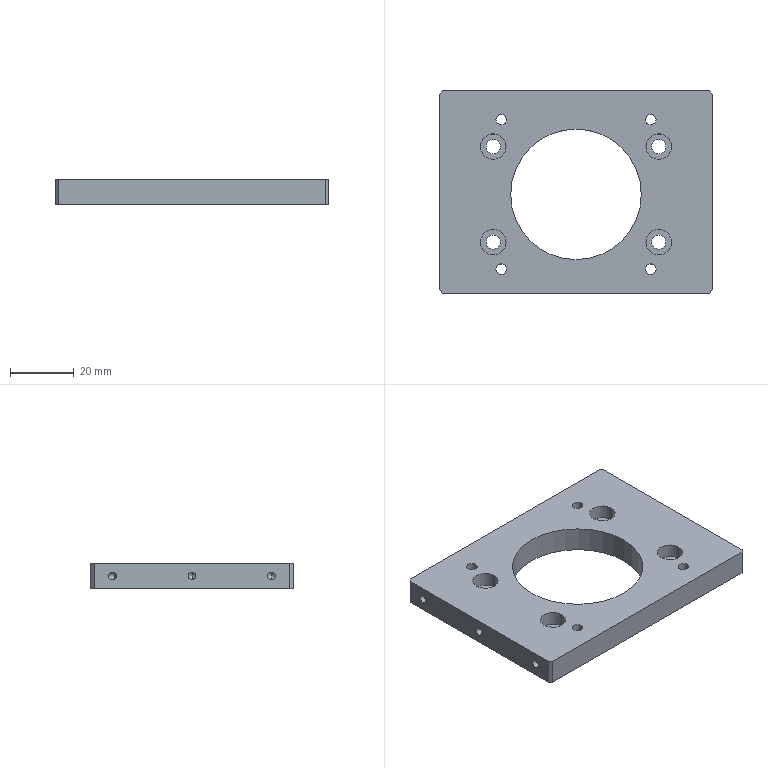Part | STEP file | KK86 stepper coupling flange | 1 solid | 76 faces | box 86 x 63.5 x 8 mm | volume 31412 mm3 | cylinder 42 | cone 20 | plane 14 | commonest cylinder face diameters 2.5 x16 3.3 x8 4.5 x8 8 x8 41 x2